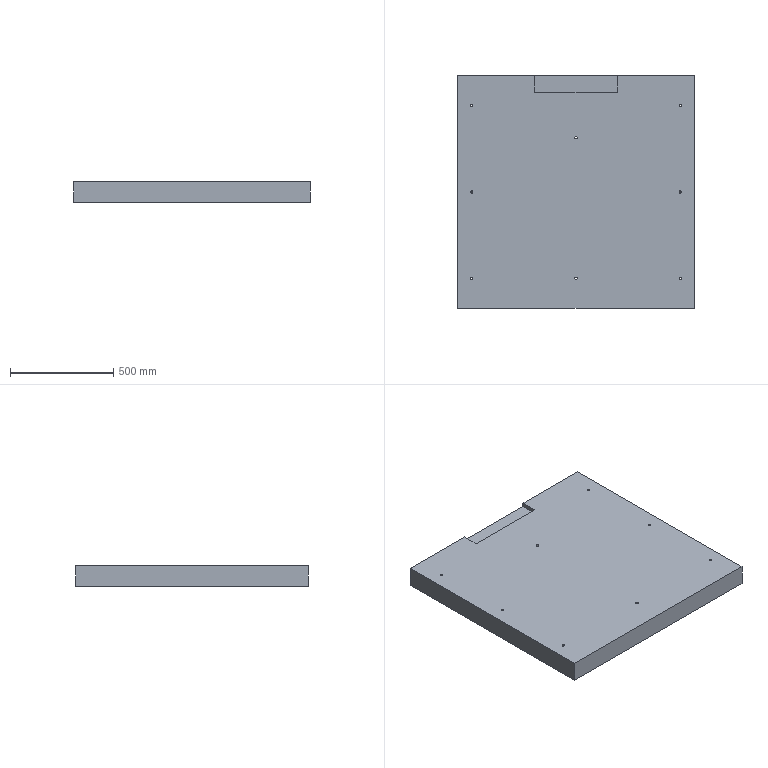Part | SolidWorks | features ICE 3, Extrusion 1 | 1 solid | 26 faces | box 1145 x 1125 x 100 mm | volume 128094667 mm3 | cylinder 16 | plane 10 | commonest cylinder face diameters 11 x14 12 x2
STEP:
#1=CARTESIAN_POINT('',(-6.,262.5,0.));
#2=VERTEX_POINT('',#1);
#3=CARTESIAN_POINT('',(6.,262.5,0.));
#4=VERTEX_POINT('',#3);
#5=CARTESIAN_POINT('',(0.,262.5,0.));
#6=DIRECTION('',(0.,0.,1.));
#7=DIRECTION('',(1.,0.,0.));
#8=AXIS2_PLACEMENT_3D('',#5,#6,#7);
#9=CIRCLE('',#8,6.);
#10=EDGE_CURVE('',#2,#4,#9,.T.);
#11=ORIENTED_EDGE('',*,*,#10,.F.);
#12=CARTESIAN_POINT('',(-6.,262.5,100.));
#13=VERTEX_POINT('',#12);
#14=CARTESIAN_POINT('',(-6.,262.5,0.));
#15=DIRECTION('',(0.,0.,1.));
#16=VECTOR('',#15,1000.);
#17=LINE('',#14,#16);
#18=EDGE_CURVE('',#2,#13,#17,.T.);
#19=ORIENTED_EDGE('',*,*,#18,.T.);
#20=CARTESIAN_POINT('',(6.,262.5,100.));
#21=VERTEX_POINT('',#20);
#22=CARTESIAN_POINT('',(0.,262.5,100.));
#23=DIRECTION('',(0.,0.,1.));
#24=DIRECTION('',(1.,0.,0.));
#25=AXIS2_PLACEMENT_3D('',#22,#23,#24);
#26=CIRCLE('',#25,6.);
#27=EDGE_CURVE('',#13,#21,#26,.T.);
#28=ORIENTED_EDGE('',*,*,#27,.T.);
#29=CARTESIAN_POINT('',(6.,262.5,0.));
#30=DIRECTION('',(0.,0.,1.));
#31=VECTOR('',#30,1000.);
#32=LINE('',#29,#31);
#33=EDGE_CURVE('',#4,#21,#32,.T.);
#34=ORIENTED_EDGE('',*,*,#33,.F.);
#35=EDGE_LOOP('',(#11,#19,#28,#34));
#36=FACE_OUTER_BOUND('',#35,.T.);
#37=CARTESIAN_POINT('',(0.,262.5,0.));
#38=DIRECTION('',(0.,0.,1.));
#39=DIRECTION('',(1.,0.,0.));
#40=AXIS2_PLACEMENT_3D('',#37,#38,#39);
#41=CYLINDRICAL_SURFACE('',#40,6.);
#42=ADVANCED_FACE('',(#36),#41,.F.);
#43=CARTESIAN_POINT('',(-5.5,-417.5,0.));
#44=VERTEX_POINT('',#43);
#45=CARTESIAN_POINT('',(5.5,-417.5,0.));
#46=VERTEX_POINT('',#45);
#47=CARTESIAN_POINT('',(0.,-417.5,0.));
#48=DIRECTION('',(0.,0.,1.));
#49=DIRECTION('',(1.,0.,0.));
#50=AXIS2_PLACEMENT_3D('',#47,#48,#49);
#51=CIRCLE('',#50,5.5);
#52=EDGE_CURVE('',#44,#46,#51,.T.);
#53=ORIENTED_EDGE('',*,*,#52,.F.);
#54=CARTESIAN_POINT('',(-5.5,-417.5,100.));
#55=VERTEX_POINT('',#54);
#56=CARTESIAN_POINT('',(-5.5,-417.5,0.));
#57=DIRECTION('',(0.,0.,1.));
#58=VECTOR('',#57,1000.);
#59=LINE('',#56,#58);
#60=EDGE_CURVE('',#44,#55,#59,.T.);
#61=ORIENTED_EDGE('',*,*,#60,.T.);
#62=CARTESIAN_POINT('',(5.5,-417.5,100.));
#63=VERTEX_POINT('',#62);
#64=CARTESIAN_POINT('',(0.,-417.5,100.));
#65=DIRECTION('',(0.,0.,1.));
#66=DIRECTION('',(1.,0.,0.));
#67=AXIS2_PLACEMENT_3D('',#64,#65,#66);
#68=CIRCLE('',#67,5.5);
#69=EDGE_CURVE('',#55,#63,#68,.T.);
#70=ORIENTED_EDGE('',*,*,#69,.T.);
#71=CARTESIAN_POINT('',(5.5,-417.5,0.));
#72=DIRECTION('',(0.,0.,1.));
#73=VECTOR('',#72,1000.);
#74=LINE('',#71,#73);
#75=EDGE_CURVE('',#46,#63,#74,.T.);
#76=ORIENTED_EDGE('',*,*,#75,.F.);
#77=EDGE_LOOP('',(#53,#61,#70,#76));
#78=FACE_OUTER_BOUND('',#77,.T.);
#79=CARTESIAN_POINT('',(0.,-417.5,0.));
#80=DIRECTION('',(0.,0.,1.));
#81=DIRECTION('',(1.,0.,0.));
#82=AXIS2_PLACEMENT_3D('',#79,#80,#81);
#83=CYLINDRICAL_SURFACE('',#82,5.5);
#84=ADVANCED_FACE('',(#78),#83,.F.);
#85=CARTESIAN_POINT('',(499.,417.5,0.));
#86=VERTEX_POINT('',#85);
#87=CARTESIAN_POINT('',(510.,417.5,0.));
#88=VERTEX_POINT('',#87);
#89=CARTESIAN_POINT('',(504.5,417.5,0.));
#90=DIRECTION('',(0.,0.,1.));
#91=DIRECTION('',(-1.,0.,0.));
#92=AXIS2_PLACEMENT_3D('',#89,#90,#91);
#93=CIRCLE('',#92,5.5);
#94=EDGE_CURVE('',#86,#88,#93,.T.);
#95=ORIENTED_EDGE('',*,*,#94,.F.);
#96=CARTESIAN_POINT('',(499.,417.5,100.));
#97=VERTEX_POINT('',#96);
#98=CARTESIAN_POINT('',(499.,417.5,0.));
#99=DIRECTION('',(0.,0.,1.));
#100=VECTOR('',#99,1000.);
#101=LINE('',#98,#100);
#102=EDGE_CURVE('',#86,#97,#101,.T.);
#103=ORIENTED_EDGE('',*,*,#102,.T.);
#104=CARTESIAN_POINT('',(510.,417.5,100.));
#105=VERTEX_POINT('',#104);
#106=CARTESIAN_POINT('',(504.5,417.5,100.));
#107=DIRECTION('',(0.,0.,1.));
#108=DIRECTION('',(1.,0.,0.));
#109=AXIS2_PLACEMENT_3D('',#106,#107,#108);
#110=CIRCLE('',#109,5.5);
#111=EDGE_CURVE('',#97,#105,#110,.T.);
#112=ORIENTED_EDGE('',*,*,#111,.T.);
#113=CARTESIAN_POINT('',(510.,417.5,0.));
#114=DIRECTION('',(0.,0.,1.));
#115=VECTOR('',#114,1000.);
#116=LINE('',#113,#115);
#117=EDGE_CURVE('',#88,#105,#116,.T.);
#118=ORIENTED_EDGE('',*,*,#117,.F.);
#119=EDGE_LOOP('',(#95,#103,#112,#118));
#120=FACE_OUTER_BOUND('',#119,.T.);
#121=CARTESIAN_POINT('',(504.5,417.5,0.));
#122=DIRECTION('',(0.,0.,1.));
#123=DIRECTION('',(1.,0.,0.));
#124=AXIS2_PLACEMENT_3D('',#121,#122,#123);
#125=CYLINDRICAL_SURFACE('',#124,5.5);
#126=ADVANCED_FACE('',(#120),#125,.F.);
#127=CARTESIAN_POINT('',(499.,-417.5,0.));
#128=VERTEX_POINT('',#127);
#129=CARTESIAN_POINT('',(510.,-417.5,0.));
#130=VERTEX_POINT('',#129);
#131=CARTESIAN_POINT('',(504.5,-417.5,0.));
#132=DIRECTION('',(0.,0.,1.));
#133=DIRECTION('',(-1.,0.,0.));
#134=AXIS2_PLACEMENT_3D('',#131,#132,#133);
#135=CIRCLE('',#134,5.5);
#136=EDGE_CURVE('',#128,#130,#135,.T.);
#137=ORIENTED_EDGE('',*,*,#136,.F.);
#138=CARTESIAN_POINT('',(499.,-417.5,100.));
#139=VERTEX_POINT('',#138);
#140=CARTESIAN_POINT('',(499.,-417.5,0.));
#141=DIRECTION('',(0.,0.,1.));
#142=VECTOR('',#141,1000.);
#143=LINE('',#140,#142);
#144=EDGE_CURVE('',#128,#139,#143,.T.);
#145=ORIENTED_EDGE('',*,*,#144,.T.);
#146=CARTESIAN_POINT('',(510.,-417.5,100.));
#147=VERTEX_POINT('',#146);
#148=CARTESIAN_POINT('',(504.5,-417.5,100.));
#149=DIRECTION('',(0.,0.,1.));
#150=DIRECTION('',(1.,0.,0.));
#151=AXIS2_PLACEMENT_3D('',#148,#149,#150);
#152=CIRCLE('',#151,5.5);
#153=EDGE_CURVE('',#139,#147,#152,.T.);
#154=ORIENTED_EDGE('',*,*,#153,.T.);
#155=CARTESIAN_POINT('',(510.,-417.5,0.));
#156=DIRECTION('',(0.,0.,1.));
#157=VECTOR('',#156,1000.);
#158=LINE('',#155,#157);
#159=EDGE_CURVE('',#130,#147,#158,.T.);
#160=ORIENTED_EDGE('',*,*,#159,.F.);
#161=EDGE_LOOP('',(#137,#145,#154,#160));
#162=FACE_OUTER_BOUND('',#161,.T.);
#163=CARTESIAN_POINT('',(504.5,-417.5,0.));
#164=DIRECTION('',(0.,0.,1.));
#165=DIRECTION('',(1.,0.,0.));
#166=AXIS2_PLACEMENT_3D('',#163,#164,#165);
#167=CYLINDRICAL_SURFACE('',#166,5.5);
#168=ADVANCED_FACE('',(#162),#167,.F.);
#169=CARTESIAN_POINT('',(-510.,-417.5,0.));
#170=VERTEX_POINT('',#169);
#171=CARTESIAN_POINT('',(-499.,-417.5,0.));
#172=VERTEX_POINT('',#171);
#173=CARTESIAN_POINT('',(-504.5,-417.5,0.));
#174=DIRECTION('',(0.,0.,1.));
#175=DIRECTION('',(1.,0.,0.));
#176=AXIS2_PLACEMENT_3D('',#173,#174,#175);
#177=CIRCLE('',#176,5.5);
#178=EDGE_CURVE('',#170,#172,#177,.T.);
#179=ORIENTED_EDGE('',*,*,#178,.F.);
#180=CARTESIAN_POINT('',(-510.,-417.5,100.));
#181=VERTEX_POINT('',#180);
#182=CARTESIAN_POINT('',(-510.,-417.5,0.));
#183=DIRECTION('',(0.,0.,1.));
#184=VECTOR('',#183,1000.);
#185=LINE('',#182,#184);
#186=EDGE_CURVE('',#170,#181,#185,.T.);
#187=ORIENTED_EDGE('',*,*,#186,.T.);
#188=CARTESIAN_POINT('',(-499.,-417.5,100.));
#189=VERTEX_POINT('',#188);
#190=CARTESIAN_POINT('',(-504.5,-417.5,100.));
#191=DIRECTION('',(0.,0.,1.));
#192=DIRECTION('',(1.,0.,0.));
#193=AXIS2_PLACEMENT_3D('',#190,#191,#192);
#194=CIRCLE('',#193,5.5);
#195=EDGE_CURVE('',#181,#189,#194,.T.);
#196=ORIENTED_EDGE('',*,*,#195,.T.);
#197=CARTESIAN_POINT('',(-499.,-417.5,0.));
#198=DIRECTION('',(0.,0.,1.));
#199=VECTOR('',#198,1000.);
#200=LINE('',#197,#199);
#201=EDGE_CURVE('',#172,#189,#200,.T.);
#202=ORIENTED_EDGE('',*,*,#201,.F.);
#203=EDGE_LOOP('',(#179,#187,#196,#202));
#204=FACE_OUTER_BOUND('',#203,.T.);
#205=CARTESIAN_POINT('',(-504.5,-417.5,0.));
#206=DIRECTION('',(0.,0.,1.));
#207=DIRECTION('',(1.,0.,0.));
#208=AXIS2_PLACEMENT_3D('',#205,#206,#207);
#209=CYLINDRICAL_SURFACE('',#208,5.5);
#210=ADVANCED_FACE('',(#204),#209,.F.);
#211=CARTESIAN_POINT('',(-510.,0.,0.));
#212=VERTEX_POINT('',#211);
#213=CARTESIAN_POINT('',(-499.,0.,0.));
#214=VERTEX_POINT('',#213);
#215=CARTESIAN_POINT('',(-504.5,0.,0.));
#216=DIRECTION('',(0.,0.,1.));
#217=DIRECTION('',(1.,0.,0.));
#218=AXIS2_PLACEMENT_3D('',#215,#216,#217);
#219=CIRCLE('',#218,5.5);
#220=EDGE_CURVE('',#212,#214,#219,.T.);
#221=ORIENTED_EDGE('',*,*,#220,.F.);
#222=CARTESIAN_POINT('',(-510.,0.,100.));
#223=VERTEX_POINT('',#222);
#224=CARTESIAN_POINT('',(-510.,0.,0.));
#225=DIRECTION('',(0.,0.,1.));
#226=VECTOR('',#225,1000.);
#227=LINE('',#224,#226);
#228=EDGE_CURVE('',#212,#223,#227,.T.);
#229=ORIENTED_EDGE('',*,*,#228,.T.);
#230=CARTESIAN_POINT('',(-499.,0.,100.));
#231=VERTEX_POINT('',#230);
#232=CARTESIAN_POINT('',(-504.5,0.,100.));
#233=DIRECTION('',(0.,0.,1.));
#234=DIRECTION('',(1.,0.,0.));
#235=AXIS2_PLACEMENT_3D('',#232,#233,#234);
#236=CIRCLE('',#235,5.5);
#237=EDGE_CURVE('',#223,#231,#236,.T.);
#238=ORIENTED_EDGE('',*,*,#237,.T.);
#239=CARTESIAN_POINT('',(-499.,0.,0.));
#240=DIRECTION('',(0.,0.,1.));
#241=VECTOR('',#240,1000.);
#242=LINE('',#239,#241);
#243=EDGE_CURVE('',#214,#231,#242,.T.);
#244=ORIENTED_EDGE('',*,*,#243,.F.);
#245=EDGE_LOOP('',(#221,#229,#238,#244));
#246=FACE_OUTER_BOUND('',#245,.T.);
#247=CARTESIAN_POINT('',(-504.5,0.,0.));
#248=DIRECTION('',(0.,0.,1.));
#249=DIRECTION('',(1.,0.,0.));
#250=AXIS2_PLACEMENT_3D('',#247,#248,#249);
#251=CYLINDRICAL_SURFACE('',#250,5.5);
#252=ADVANCED_FACE('',(#246),#251,.F.);
#253=CARTESIAN_POINT('',(499.,0.,0.));
#254=VERTEX_POINT('',#253);
#255=CARTESIAN_POINT('',(510.,0.,0.));
#256=VERTEX_POINT('',#255);
#257=CARTESIAN_POINT('',(504.5,0.,0.));
#258=DIRECTION('',(0.,0.,1.));
#259=DIRECTION('',(-1.,0.,0.));
#260=AXIS2_PLACEMENT_3D('',#257,#258,#259);
#261=CIRCLE('',#260,5.5);
#262=EDGE_CURVE('',#254,#256,#261,.T.);
#263=ORIENTED_EDGE('',*,*,#262,.F.);
#264=CARTESIAN_POINT('',(499.,0.,100.));
#265=VERTEX_POINT('',#264);
#266=CARTESIAN_POINT('',(499.,0.,0.));
#267=DIRECTION('',(0.,0.,1.));
#268=VECTOR('',#267,1000.);
#269=LINE('',#266,#268);
#270=EDGE_CURVE('',#254,#265,#269,.T.);
#271=ORIENTED_EDGE('',*,*,#270,.T.);
#272=CARTESIAN_POINT('',(510.,0.,100.));
#273=VERTEX_POINT('',#272);
#274=CARTESIAN_POINT('',(504.5,0.,100.));
#275=DIRECTION('',(0.,0.,1.));
#276=DIRECTION('',(1.,0.,0.));
#277=AXIS2_PLACEMENT_3D('',#274,#275,#276);
#278=CIRCLE('',#277,5.5);
#279=EDGE_CURVE('',#265,#273,#278,.T.);
#280=ORIENTED_EDGE('',*,*,#279,.T.);
#281=CARTESIAN_POINT('',(510.,0.,0.));
#282=DIRECTION('',(0.,0.,1.));
#283=VECTOR('',#282,1000.);
#284=LINE('',#281,#283);
#285=EDGE_CURVE('',#256,#273,#284,.T.);
#286=ORIENTED_EDGE('',*,*,#285,.F.);
#287=EDGE_LOOP('',(#263,#271,#280,#286));
#288=FACE_OUTER_BOUND('',#287,.T.);
#289=CARTESIAN_POINT('',(504.5,0.,0.));
#290=DIRECTION('',(0.,0.,1.));
#291=DIRECTION('',(1.,0.,0.));
#292=AXIS2_PLACEMENT_3D('',#289,#290,#291);
#293=CYLINDRICAL_SURFACE('',#292,5.5);
#294=ADVANCED_FACE('',(#288),#293,.F.);
#295=CARTESIAN_POINT('',(-510.,417.5,0.));
#296=VERTEX_POINT('',#295);
#297=CARTESIAN_POINT('',(-499.,417.5,0.));
#298=VERTEX_POINT('',#297);
#299=CARTESIAN_POINT('',(-504.5,417.5,0.));
#300=DIRECTION('',(0.,0.,1.));
#301=DIRECTION('',(1.,0.,0.));
#302=AXIS2_PLACEMENT_3D('',#299,#300,#301);
#303=CIRCLE('',#302,5.5);
#304=EDGE_CURVE('',#296,#298,#303,.T.);
#305=ORIENTED_EDGE('',*,*,#304,.F.);
#306=CARTESIAN_POINT('',(-510.,417.5,100.));
#307=VERTEX_POINT('',#306);
#308=CARTESIAN_POINT('',(-510.,417.5,0.));
#309=DIRECTION('',(0.,0.,1.));
#310=VECTOR('',#309,1000.);
#311=LINE('',#308,#310);
#312=EDGE_CURVE('',#296,#307,#311,.T.);
#313=ORIENTED_EDGE('',*,*,#312,.T.);
#314=CARTESIAN_POINT('',(-499.,417.5,100.));
#315=VERTEX_POINT('',#314);
#316=CARTESIAN_POINT('',(-504.5,417.5,100.));
#317=DIRECTION('',(0.,0.,1.));
#318=DIRECTION('',(1.,0.,0.));
#319=AXIS2_PLACEMENT_3D('',#316,#317,#318);
#320=CIRCLE('',#319,5.5);
#321=EDGE_CURVE('',#307,#315,#320,.T.);
#322=ORIENTED_EDGE('',*,*,#321,.T.);
#323=CARTESIAN_POINT('',(-499.,417.5,0.));
#324=DIRECTION('',(0.,0.,1.));
#325=VECTOR('',#324,1000.);
#326=LINE('',#323,#325);
#327=EDGE_CURVE('',#298,#315,#326,.T.);
#328=ORIENTED_EDGE('',*,*,#327,.F.);
#329=EDGE_LOOP('',(#305,#313,#322,#328));
#330=FACE_OUTER_BOUND('',#329,.T.);
#331=CARTESIAN_POINT('',(-504.5,417.5,0.));
#332=DIRECTION('',(0.,0.,1.));
#333=DIRECTION('',(1.,0.,0.));
#334=AXIS2_PLACEMENT_3D('',#331,#332,#333);
#335=CYLINDRICAL_SURFACE('',#334,5.5);
#336=ADVANCED_FACE('',(#330),#335,.F.);
#337=CARTESIAN_POINT('',(572.5,-562.5,0.));
#338=VERTEX_POINT('',#337);
#339=CARTESIAN_POINT('',(572.5,562.5,0.));
#340=VERTEX_POINT('',#339);
#341=CARTESIAN_POINT('',(572.5,562.5,0.));
#342=DIRECTION('',(0.,1.,0.));
#343=VECTOR('',#342,1000.);
#344=LINE('',#341,#343);
#345=EDGE_CURVE('',#338,#340,#344,.T.);
#346=ORIENTED_EDGE('',*,*,#345,.T.);
#347=CARTESIAN_POINT('',(572.5,562.5,100.));
#348=VERTEX_POINT('',#347);
#349=CARTESIAN_POINT('',(572.5,562.5,100.));
#350=DIRECTION('',(0.,0.,-1.));
#351=VECTOR('',#350,1000.);
#352=LINE('',#349,#351);
#353=EDGE_CURVE('',#348,#340,#352,.T.);
#354=ORIENTED_EDGE('',*,*,#353,.F.);
#355=CARTESIAN_POINT('',(572.5,-562.5,100.));
#356=VERTEX_POINT('',#355);
#357=CARTESIAN_POINT('',(572.5,562.5,100.));
#358=DIRECTION('',(0.,1.,0.));
#359=VECTOR('',#358,1000.);
#360=LINE('',#357,#359);
#361=EDGE_CURVE('',#356,#348,#360,.T.);
#362=ORIENTED_EDGE('',*,*,#361,.F.);
#363=CARTESIAN_POINT('',(572.5,-562.5,100.));
#364=DIRECTION('',(0.,0.,-1.));
#365=VECTOR('',#364,1000.);
#366=LINE('',#363,#365);
#367=EDGE_CURVE('',#356,#338,#366,.T.);
#368=ORIENTED_EDGE('',*,*,#367,.T.);
#369=EDGE_LOOP('',(#346,#354,#362,#368));
#370=FACE_OUTER_BOUND('',#369,.T.);
#371=CARTESIAN_POINT('',(572.5,562.5,100.));
#372=DIRECTION('',(-1.,0.,0.));
#373=DIRECTION('',(0.,-1.,0.));
#374=AXIS2_PLACEMENT_3D('',#371,#372,#373);
#375=PLANE('',#374);
#376=ADVANCED_FACE('',(#370),#375,.F.);
#377=CARTESIAN_POINT('',(200.,562.5,80.));
#378=VERTEX_POINT('',#377);
#379=CARTESIAN_POINT('',(-200.,562.5,80.));
#380=VERTEX_POINT('',#379);
#381=CARTESIAN_POINT('',(-572.5,562.5,80.));
#382=DIRECTION('',(-1.,0.,0.));
#383=VECTOR('',#382,1000.);
#384=LINE('',#381,#383);
#385=EDGE_CURVE('',#378,#380,#384,.T.);
#386=ORIENTED_EDGE('',*,*,#385,.F.);
#387=CARTESIAN_POINT('',(200.,562.5,100.));
#388=VERTEX_POINT('',#387);
#389=CARTESIAN_POINT('',(200.,562.5,100.));
#390=DIRECTION('',(0.,0.,1.));
#391=VECTOR('',#390,1000.);
#392=LINE('',#389,#391);
#393=EDGE_CURVE('',#378,#388,#392,.T.);
#394=ORIENTED_EDGE('',*,*,#393,.T.);
#395=CARTESIAN_POINT('',(-572.5,562.5,100.));
#396=DIRECTION('',(-1.,0.,0.));
#397=VECTOR('',#396,1000.);
#398=LINE('',#395,#397);
#399=EDGE_CURVE('',#348,#388,#398,.T.);
#400=ORIENTED_EDGE('',*,*,#399,.F.);
#401=ORIENTED_EDGE('',*,*,#353,.T.);
#402=CARTESIAN_POINT('',(-572.5,562.5,0.));
#403=VERTEX_POINT('',#402);
#404=CARTESIAN_POINT('',(-572.5,562.5,0.));
#405=DIRECTION('',(-1.,0.,0.));
#406=VECTOR('',#405,1000.);
#407=LINE('',#404,#406);
#408=EDGE_CURVE('',#340,#403,#407,.T.);
#409=ORIENTED_EDGE('',*,*,#408,.T.);
#410=CARTESIAN_POINT('',(-572.5,562.5,100.));
#411=VERTEX_POINT('',#410);
#412=CARTESIAN_POINT('',(-572.5,562.5,100.));
#413=DIRECTION('',(0.,0.,-1.));
#414=VECTOR('',#413,1000.);
#415=LINE('',#412,#414);
#416=EDGE_CURVE('',#411,#403,#415,.T.);
#417=ORIENTED_EDGE('',*,*,#416,.F.);
#418=CARTESIAN_POINT('',(-200.,562.5,100.));
#419=VERTEX_POINT('',#418);
#420=CARTESIAN_POINT('',(-572.5,562.5,100.));
#421=DIRECTION('',(-1.,0.,0.));
#422=VECTOR('',#421,1000.);
#423=LINE('',#420,#422);
#424=EDGE_CURVE('',#419,#411,#423,.T.);
#425=ORIENTED_EDGE('',*,*,#424,.F.);
#426=CARTESIAN_POINT('',(-200.,562.5,100.));
#427=DIRECTION('',(0.,0.,-1.));
#428=VECTOR('',#427,1000.);
#429=LINE('',#426,#428);
#430=EDGE_CURVE('',#419,#380,#429,.T.);
#431=ORIENTED_EDGE('',*,*,#430,.T.);
#432=EDGE_LOOP('',(#386,#394,#400,#401,#409,#417,#425,#431));
#433=FACE_OUTER_BOUND('',#432,.T.);
#434=CARTESIAN_POINT('',(-572.5,562.5,100.));
#435=DIRECTION('',(0.,-1.,0.));
#436=DIRECTION('',(0.,0.,-1.));
#437=AXIS2_PLACEMENT_3D('',#434,#435,#436);
#438=PLANE('',#437);
#439=ADVANCED_FACE('',(#433),#438,.F.);
#440=CARTESIAN_POINT('',(-572.5,-562.5,0.));
#441=VERTEX_POINT('',#440);
#442=CARTESIAN_POINT('',(-572.5,562.5,0.));
#443=DIRECTION('',(0.,-1.,0.));
#444=VECTOR('',#443,1000.);
#445=LINE('',#442,#444);
#446=EDGE_CURVE('',#403,#441,#445,.T.);
#447=ORIENTED_EDGE('',*,*,#446,.T.);
#448=CARTESIAN_POINT('',(-572.5,-562.5,100.));
#449=VERTEX_POINT('',#448);
#450=CARTESIAN_POINT('',(-572.5,-562.5,100.));
#451=DIRECTION('',(0.,0.,-1.));
#452=VECTOR('',#451,1000.);
#453=LINE('',#450,#452);
#454=EDGE_CURVE('',#449,#441,#453,.T.);
#455=ORIENTED_EDGE('',*,*,#454,.F.);
#456=CARTESIAN_POINT('',(-572.5,562.5,100.));
#457=DIRECTION('',(0.,-1.,0.));
#458=VECTOR('',#457,1000.);
#459=LINE('',#456,#458);
#460=EDGE_CURVE('',#411,#449,#459,.T.);
#461=ORIENTED_EDGE('',*,*,#460,.F.);
#462=ORIENTED_EDGE('',*,*,#416,.T.);
#463=EDGE_LOOP('',(#447,#455,#461,#462));
#464=FACE_OUTER_BOUND('',#463,.T.);
#465=CARTESIAN_POINT('',(-572.5,562.5,100.));
#466=DIRECTION('',(1.,0.,0.));
#467=DIRECTION('',(0.,1.,0.));
#468=AXIS2_PLACEMENT_3D('',#465,#466,#467);
#469=PLANE('',#468);
#470=ADVANCED_FACE('',(#464),#469,.F.);
#471=CARTESIAN_POINT('',(-572.5,-562.5,0.));
#472=DIRECTION('',(1.,0.,0.));
#473=VECTOR('',#472,1000.);
#474=LINE('',#471,#473);
#475=EDGE_CURVE('',#441,#338,#474,.T.);
#476=ORIENTED_EDGE('',*,*,#475,.T.);
#477=ORIENTED_EDGE('',*,*,#367,.F.);
#478=CARTESIAN_POINT('',(-572.5,-562.5,100.));
#479=DIRECTION('',(1.,0.,0.));
#480=VECTOR('',#479,1000.);
#481=LINE('',#478,#480);
#482=EDGE_CURVE('',#449,#356,#481,.T.);
#483=ORIENTED_EDGE('',*,*,#482,.F.);
#484=ORIENTED_EDGE('',*,*,#454,.T.);
#485=EDGE_LOOP('',(#476,#477,#483,#484));
#486=FACE_OUTER_BOUND('',#485,.T.);
#487=CARTESIAN_POINT('',(-572.5,-562.5,100.));
#488=DIRECTION('',(0.,1.,0.));
#489=DIRECTION('',(0.,0.,1.));
#490=AXIS2_PLACEMENT_3D('',#487,#488,#489);
#491=PLANE('',#490);
#492=ADVANCED_FACE('',(#486),#491,.F.);
#493=CARTESIAN_POINT('',(0.,262.5,100.));
#494=DIRECTION('',(0.,0.,1.));
#495=DIRECTION('',(1.,0.,0.));
#496=AXIS2_PLACEMENT_3D('',#493,#494,#495);
#497=CIRCLE('',#496,6.);
#498=EDGE_CURVE('',#21,#13,#497,.T.);
#499=ORIENTED_EDGE('',*,*,#498,.F.);
#500=ORIENTED_EDGE('',*,*,#27,.F.);
#501=EDGE_LOOP('',(#499,#500));
#502=FACE_BOUND('',#501,.T.);
#503=CARTESIAN_POINT('',(0.,-417.5,100.));
#504=DIRECTION('',(0.,0.,1.));
#505=DIRECTION('',(1.,0.,0.));
#506=AXIS2_PLACEMENT_3D('',#503,#504,#505);
#507=CIRCLE('',#506,5.5);
#508=EDGE_CURVE('',#63,#55,#507,.T.);
#509=ORIENTED_EDGE('',*,*,#508,.F.);
#510=ORIENTED_EDGE('',*,*,#69,.F.);
#511=EDGE_LOOP('',(#509,#510));
#512=FACE_BOUND('',#511,.T.);
#513=CARTESIAN_POINT('',(504.5,417.5,100.));
#514=DIRECTION('',(0.,0.,1.));
#515=DIRECTION('',(1.,0.,0.));
#516=AXIS2_PLACEMENT_3D('',#513,#514,#515);
#517=CIRCLE('',#516,5.5);
#518=EDGE_CURVE('',#105,#97,#517,.T.);
#519=ORIENTED_EDGE('',*,*,#518,.F.);
#520=ORIENTED_EDGE('',*,*,#111,.F.);
#521=EDGE_LOOP('',(#519,#520));
#522=FACE_BOUND('',#521,.T.);
#523=CARTESIAN_POINT('',(504.5,-417.5,100.));
#524=DIRECTION('',(0.,0.,1.));
#525=DIRECTION('',(1.,0.,0.));
#526=AXIS2_PLACEMENT_3D('',#523,#524,#525);
#527=CIRCLE('',#526,5.5);
#528=EDGE_CURVE('',#147,#139,#527,.T.);
#529=ORIENTED_EDGE('',*,*,#528,.F.);
#530=ORIENTED_EDGE('',*,*,#153,.F.);
#531=EDGE_LOOP('',(#529,#530));
#532=FACE_BOUND('',#531,.T.);
#533=CARTESIAN_POINT('',(-504.5,-417.5,100.));
#534=DIRECTION('',(0.,0.,1.));
#535=DIRECTION('',(1.,0.,0.));
#536=AXIS2_PLACEMENT_3D('',#533,#534,#535);
#537=CIRCLE('',#536,5.5);
#538=EDGE_CURVE('',#189,#181,#537,.T.);
#539=ORIENTED_EDGE('',*,*,#538,.F.);
#540=ORIENTED_EDGE('',*,*,#195,.F.);
#541=EDGE_LOOP('',(#539,#540));
#542=FACE_BOUND('',#541,.T.);
#543=CARTESIAN_POINT('',(-504.5,0.,100.));
#544=DIRECTION('',(0.,0.,1.));
#545=DIRECTION('',(1.,0.,0.));
#546=AXIS2_PLACEMENT_3D('',#543,#544,#545);
#547=CIRCLE('',#546,5.5);
#548=EDGE_CURVE('',#231,#223,#547,.T.);
#549=ORIENTED_EDGE('',*,*,#548,.F.);
#550=ORIENTED_EDGE('',*,*,#237,.F.);
#551=EDGE_LOOP('',(#549,#550));
#552=FACE_BOUND('',#551,.T.);
#553=CARTESIAN_POINT('',(504.5,0.,100.));
#554=DIRECTION('',(0.,0.,1.));
#555=DIRECTION('',(1.,0.,0.));
#556=AXIS2_PLACEMENT_3D('',#553,#554,#555);
#557=CIRCLE('',#556,5.5);
#558=EDGE_CURVE('',#273,#265,#557,.T.);
#559=ORIENTED_EDGE('',*,*,#558,.F.);
#560=ORIENTED_EDGE('',*,*,#279,.F.);
#561=EDGE_LOOP('',(#559,#560));
#562=FACE_BOUND('',#561,.T.);
#563=CARTESIAN_POINT('',(-504.5,417.5,100.));
#564=DIRECTION('',(0.,0.,1.));
#565=DIRECTION('',(1.,0.,0.));
#566=AXIS2_PLACEMENT_3D('',#563,#564,#565);
#567=CIRCLE('',#566,5.5);
#568=EDGE_CURVE('',#315,#307,#567,.T.);
#569=ORIENTED_EDGE('',*,*,#568,.F.);
#570=ORIENTED_EDGE('',*,*,#321,.F.);
#571=EDGE_LOOP('',(#569,#570));
#572=FACE_BOUND('',#571,.T.);
#573=CARTESIAN_POINT('',(200.,482.5,100.));
#574=VERTEX_POINT('',#573);
#575=CARTESIAN_POINT('',(200.,642.5,100.));
#576=DIRECTION('',(0.,1.,0.));
#577=VECTOR('',#576,1000.);
#578=LINE('',#575,#577);
#579=EDGE_CURVE('',#574,#388,#578,.T.);
#580=ORIENTED_EDGE('',*,*,#579,.F.);
#581=CARTESIAN_POINT('',(-200.,482.5,100.));
#582=VERTEX_POINT('',#581);
#583=CARTESIAN_POINT('',(-200.,482.5,100.));
#584=DIRECTION('',(1.,0.,0.));
#585=VECTOR('',#584,1000.);
#586=LINE('',#583,#585);
#587=EDGE_CURVE('',#582,#574,#586,.T.);
#588=ORIENTED_EDGE('',*,*,#587,.F.);
#589=CARTESIAN_POINT('',(-200.,0.,100.));
#590=DIRECTION('',(0.,-1.,0.));
#591=VECTOR('',#590,1000.);
#592=LINE('',#589,#591);
#593=EDGE_CURVE('',#419,#582,#592,.T.);
#594=ORIENTED_EDGE('',*,*,#593,.F.);
#595=ORIENTED_EDGE('',*,*,#424,.T.);
#596=ORIENTED_EDGE('',*,*,#460,.T.);
#597=ORIENTED_EDGE('',*,*,#482,.T.);
#598=ORIENTED_EDGE('',*,*,#361,.T.);
#599=ORIENTED_EDGE('',*,*,#399,.T.);
#600=EDGE_LOOP('',(#580,#588,#594,#595,#596,#597,#598,#599));
#601=FACE_OUTER_BOUND('',#600,.T.);
#602=CARTESIAN_POINT('',(0.,0.,100.));
#603=DIRECTION('',(0.,0.,1.));
#604=DIRECTION('',(1.,0.,0.));
#605=AXIS2_PLACEMENT_3D('',#602,#603,#604);
#606=PLANE('',#605);
#607=ADVANCED_FACE('',(#502,#512,#522,#532,#542,#552,#562,#572,#601),#606,.T.);
#608=CARTESIAN_POINT('',(0.,262.5,0.));
#609=DIRECTION('',(0.,0.,1.));
#610=DIRECTION('',(1.,0.,0.));
#611=AXIS2_PLACEMENT_3D('',#608,#609,#610);
#612=CIRCLE('',#611,6.);
#613=EDGE_CURVE('',#4,#2,#612,.T.);
#614=ORIENTED_EDGE('',*,*,#613,.T.);
#615=ORIENTED_EDGE('',*,*,#10,.T.);
#616=EDGE_LOOP('',(#614,#615));
#617=FACE_BOUND('',#616,.T.);
#618=CARTESIAN_POINT('',(0.,-417.5,0.));
#619=DIRECTION('',(0.,0.,1.));
#620=DIRECTION('',(1.,0.,0.));
#621=AXIS2_PLACEMENT_3D('',#618,#619,#620);
#622=CIRCLE('',#621,5.5);
#623=EDGE_CURVE('',#46,#44,#622,.T.);
#624=ORIENTED_EDGE('',*,*,#623,.T.);
#625=ORIENTED_EDGE('',*,*,#52,.T.);
#626=EDGE_LOOP('',(#624,#625));
#627=FACE_BOUND('',#626,.T.);
#628=CARTESIAN_POINT('',(504.5,417.5,0.));
#629=DIRECTION('',(0.,0.,1.));
#630=DIRECTION('',(-1.,0.,0.));
#631=AXIS2_PLACEMENT_3D('',#628,#629,#630);
#632=CIRCLE('',#631,5.5);
#633=EDGE_CURVE('',#88,#86,#632,.T.);
#634=ORIENTED_EDGE('',*,*,#633,.T.);
#635=ORIENTED_EDGE('',*,*,#94,.T.);
#636=EDGE_LOOP('',(#634,#635));
#637=FACE_BOUND('',#636,.T.);
#638=CARTESIAN_POINT('',(504.5,-417.5,0.));
#639=DIRECTION('',(0.,0.,1.));
#640=DIRECTION('',(-1.,0.,0.));
#641=AXIS2_PLACEMENT_3D('',#638,#639,#640);
#642=CIRCLE('',#641,5.5);
#643=EDGE_CURVE('',#130,#128,#642,.T.);
#644=ORIENTED_EDGE('',*,*,#643,.T.);
#645=ORIENTED_EDGE('',*,*,#136,.T.);
#646=EDGE_LOOP('',(#644,#645));
#647=FACE_BOUND('',#646,.T.);
#648=CARTESIAN_POINT('',(-504.5,-417.5,0.));
#649=DIRECTION('',(0.,0.,1.));
#650=DIRECTION('',(1.,0.,0.));
#651=AXIS2_PLACEMENT_3D('',#648,#649,#650);
#652=CIRCLE('',#651,5.5);
#653=EDGE_CURVE('',#172,#170,#652,.T.);
#654=ORIENTED_EDGE('',*,*,#653,.T.);
#655=ORIENTED_EDGE('',*,*,#178,.T.);
#656=EDGE_LOOP('',(#654,#655));
#657=FACE_BOUND('',#656,.T.);
#658=CARTESIAN_POINT('',(-504.5,0.,0.));
#659=DIRECTION('',(0.,0.,1.));
#660=DIRECTION('',(1.,0.,0.));
#661=AXIS2_PLACEMENT_3D('',#658,#659,#660);
#662=CIRCLE('',#661,5.5);
#663=EDGE_CURVE('',#214,#212,#662,.T.);
#664=ORIENTED_EDGE('',*,*,#663,.T.);
#665=ORIENTED_EDGE('',*,*,#220,.T.);
#666=EDGE_LOOP('',(#664,#665));
#667=FACE_BOUND('',#666,.T.);
#668=CARTESIAN_POINT('',(504.5,0.,0.));
#669=DIRECTION('',(0.,0.,1.));
#670=DIRECTION('',(-1.,0.,0.));
#671=AXIS2_PLACEMENT_3D('',#668,#669,#670);
#672=CIRCLE('',#671,5.5);
#673=EDGE_CURVE('',#256,#254,#672,.T.);
#674=ORIENTED_EDGE('',*,*,#673,.T.);
#675=ORIENTED_EDGE('',*,*,#262,.T.);
#676=EDGE_LOOP('',(#674,#675));
#677=FACE_BOUND('',#676,.T.);
#678=CARTESIAN_POINT('',(-504.5,417.5,0.));
#679=DIRECTION('',(0.,0.,1.));
#680=DIRECTION('',(1.,0.,0.));
#681=AXIS2_PLACEMENT_3D('',#678,#679,#680);
#682=CIRCLE('',#681,5.5);
#683=EDGE_CURVE('',#298,#296,#682,.T.);
#684=ORIENTED_EDGE('',*,*,#683,.T.);
#685=ORIENTED_EDGE('',*,*,#304,.T.);
#686=EDGE_LOOP('',(#684,#685));
#687=FACE_BOUND('',#686,.T.);
#688=ORIENTED_EDGE('',*,*,#345,.F.);
#689=ORIENTED_EDGE('',*,*,#475,.F.);
#690=ORIENTED_EDGE('',*,*,#446,.F.);
#691=ORIENTED_EDGE('',*,*,#408,.F.);
#692=EDGE_LOOP('',(#688,#689,#690,#691));
#693=FACE_OUTER_BOUND('',#692,.T.);
#694=CARTESIAN_POINT('',(0.,0.,0.));
#695=DIRECTION('',(0.,0.,1.));
#696=DIRECTION('',(1.,0.,0.));
#697=AXIS2_PLACEMENT_3D('',#694,#695,#696);
#698=PLANE('',#697);
#699=ADVANCED_FACE('',(#617,#627,#637,#647,#657,#667,#677,#687,#693),#698,.F.);
#700=ORIENTED_EDGE('',*,*,#385,.T.);
#701=CARTESIAN_POINT('',(-200.,482.5,80.));
#702=VERTEX_POINT('',#701);
#703=CARTESIAN_POINT('',(-200.,642.5,80.));
#704=DIRECTION('',(0.,-1.,0.));
#705=VECTOR('',#704,1000.);
#706=LINE('',#703,#705);
#707=EDGE_CURVE('',#380,#702,#706,.T.);
#708=ORIENTED_EDGE('',*,*,#707,.T.);
#709=CARTESIAN_POINT('',(200.,482.5,80.));
#710=VERTEX_POINT('',#709);
#711=CARTESIAN_POINT('',(-200.,482.5,80.));
#712=DIRECTION('',(1.,0.,0.));
#713=VECTOR('',#712,1000.);
#714=LINE('',#711,#713);
#715=EDGE_CURVE('',#702,#710,#714,.T.);
#716=ORIENTED_EDGE('',*,*,#715,.T.);
#717=CARTESIAN_POINT('',(200.,642.5,80.));
#718=DIRECTION('',(0.,1.,0.));
#719=VECTOR('',#718,1000.);
#720=LINE('',#717,#719);
#721=EDGE_CURVE('',#710,#378,#720,.T.);
#722=ORIENTED_EDGE('',*,*,#721,.T.);
#723=EDGE_LOOP('',(#700,#708,#716,#722));
#724=FACE_OUTER_BOUND('',#723,.T.);
#725=CARTESIAN_POINT('',(0.,0.,80.));
#726=DIRECTION('',(0.,0.,1.));
#727=DIRECTION('',(1.,0.,0.));
#728=AXIS2_PLACEMENT_3D('',#725,#726,#727);
#729=PLANE('',#728);
#730=ADVANCED_FACE('',(#724),#729,.T.);
#731=ORIENTED_EDGE('',*,*,#721,.F.);
#732=CARTESIAN_POINT('',(200.,482.5,80.));
#733=DIRECTION('',(0.,0.,1.));
#734=VECTOR('',#733,1000.);
#735=LINE('',#732,#734);
#736=EDGE_CURVE('',#710,#574,#735,.T.);
#737=ORIENTED_EDGE('',*,*,#736,.T.);
#738=ORIENTED_EDGE('',*,*,#579,.T.);
#739=ORIENTED_EDGE('',*,*,#393,.F.);
#740=EDGE_LOOP('',(#731,#737,#738,#739));
#741=FACE_OUTER_BOUND('',#740,.T.);
#742=CARTESIAN_POINT('',(200.,642.5,80.));
#743=DIRECTION('',(1.,0.,0.));
#744=DIRECTION('',(0.,1.,0.));
#745=AXIS2_PLACEMENT_3D('',#742,#743,#744);
#746=PLANE('',#745);
#747=ADVANCED_FACE('',(#741),#746,.F.);
#748=ORIENTED_EDGE('',*,*,#593,.T.);
#749=CARTESIAN_POINT('',(-200.,482.5,80.));
#750=DIRECTION('',(0.,0.,1.));
#751=VECTOR('',#750,1000.);
#752=LINE('',#749,#751);
#753=EDGE_CURVE('',#702,#582,#752,.T.);
#754=ORIENTED_EDGE('',*,*,#753,.F.);
#755=ORIENTED_EDGE('',*,*,#707,.F.);
#756=ORIENTED_EDGE('',*,*,#430,.F.);
#757=EDGE_LOOP('',(#748,#754,#755,#756));
#758=FACE_OUTER_BOUND('',#757,.T.);
#759=CARTESIAN_POINT('',(-200.,642.5,80.));
#760=DIRECTION('',(-1.,0.,0.));
#761=DIRECTION('',(0.,0.,1.));
#762=AXIS2_PLACEMENT_3D('',#759,#760,#761);
#763=PLANE('',#762);
#764=ADVANCED_FACE('',(#758),#763,.F.);
#765=ORIENTED_EDGE('',*,*,#587,.T.);
#766=ORIENTED_EDGE('',*,*,#736,.F.);
#767=ORIENTED_EDGE('',*,*,#715,.F.);
#768=ORIENTED_EDGE('',*,*,#753,.T.);
#769=EDGE_LOOP('',(#765,#766,#767,#768));
#770=FACE_OUTER_BOUND('',#769,.T.);
#771=CARTESIAN_POINT('',(-200.,482.5,80.));
#772=DIRECTION('',(0.,-1.,0.));
#773=DIRECTION('',(0.,0.,-1.));
#774=AXIS2_PLACEMENT_3D('',#771,#772,#773);
#775=PLANE('',#774);
#776=ADVANCED_FACE('',(#770),#775,.F.);
#777=ORIENTED_EDGE('',*,*,#312,.F.);
#778=ORIENTED_EDGE('',*,*,#683,.F.);
#779=ORIENTED_EDGE('',*,*,#327,.T.);
#780=ORIENTED_EDGE('',*,*,#568,.T.);
#781=EDGE_LOOP('',(#777,#778,#779,#780));
#782=FACE_OUTER_BOUND('',#781,.T.);
#783=CARTESIAN_POINT('',(-504.5,417.5,0.));
#784=DIRECTION('',(0.,0.,1.));
#785=DIRECTION('',(1.,0.,0.));
#786=AXIS2_PLACEMENT_3D('',#783,#784,#785);
#787=CYLINDRICAL_SURFACE('',#786,5.5);
#788=ADVANCED_FACE('',(#782),#787,.F.);
#789=ORIENTED_EDGE('',*,*,#270,.F.);
#790=ORIENTED_EDGE('',*,*,#673,.F.);
#791=ORIENTED_EDGE('',*,*,#285,.T.);
#792=ORIENTED_EDGE('',*,*,#558,.T.);
#793=EDGE_LOOP('',(#789,#790,#791,#792));
#794=FACE_OUTER_BOUND('',#793,.T.);
#795=CARTESIAN_POINT('',(504.5,0.,0.));
#796=DIRECTION('',(0.,0.,1.));
#797=DIRECTION('',(1.,0.,0.));
#798=AXIS2_PLACEMENT_3D('',#795,#796,#797);
#799=CYLINDRICAL_SURFACE('',#798,5.5);
#800=ADVANCED_FACE('',(#794),#799,.F.);
#801=ORIENTED_EDGE('',*,*,#228,.F.);
#802=ORIENTED_EDGE('',*,*,#663,.F.);
#803=ORIENTED_EDGE('',*,*,#243,.T.);
#804=ORIENTED_EDGE('',*,*,#548,.T.);
#805=EDGE_LOOP('',(#801,#802,#803,#804));
#806=FACE_OUTER_BOUND('',#805,.T.);
#807=CARTESIAN_POINT('',(-504.5,0.,0.));
#808=DIRECTION('',(0.,0.,1.));
#809=DIRECTION('',(1.,0.,0.));
#810=AXIS2_PLACEMENT_3D('',#807,#808,#809);
#811=CYLINDRICAL_SURFACE('',#810,5.5);
#812=ADVANCED_FACE('',(#806),#811,.F.);
#813=ORIENTED_EDGE('',*,*,#186,.F.);
#814=ORIENTED_EDGE('',*,*,#653,.F.);
#815=ORIENTED_EDGE('',*,*,#201,.T.);
#816=ORIENTED_EDGE('',*,*,#538,.T.);
#817=EDGE_LOOP('',(#813,#814,#815,#816));
#818=FACE_OUTER_BOUND('',#817,.T.);
#819=CARTESIAN_POINT('',(-504.5,-417.5,0.));
#820=DIRECTION('',(0.,0.,1.));
#821=DIRECTION('',(1.,0.,0.));
#822=AXIS2_PLACEMENT_3D('',#819,#820,#821);
#823=CYLINDRICAL_SURFACE('',#822,5.5);
#824=ADVANCED_FACE('',(#818),#823,.F.);
#825=ORIENTED_EDGE('',*,*,#144,.F.);
#826=ORIENTED_EDGE('',*,*,#643,.F.);
#827=ORIENTED_EDGE('',*,*,#159,.T.);
#828=ORIENTED_EDGE('',*,*,#528,.T.);
#829=EDGE_LOOP('',(#825,#826,#827,#828));
#830=FACE_OUTER_BOUND('',#829,.T.);
#831=CARTESIAN_POINT('',(504.5,-417.5,0.));
#832=DIRECTION('',(0.,0.,1.));
#833=DIRECTION('',(1.,0.,0.));
#834=AXIS2_PLACEMENT_3D('',#831,#832,#833);
#835=CYLINDRICAL_SURFACE('',#834,5.5);
#836=ADVANCED_FACE('',(#830),#835,.F.);
#837=ORIENTED_EDGE('',*,*,#102,.F.);
#838=ORIENTED_EDGE('',*,*,#633,.F.);
#839=ORIENTED_EDGE('',*,*,#117,.T.);
#840=ORIENTED_EDGE('',*,*,#518,.T.);
#841=EDGE_LOOP('',(#837,#838,#839,#840));
#842=FACE_OUTER_BOUND('',#841,.T.);
#843=CARTESIAN_POINT('',(504.5,417.5,0.));
#844=DIRECTION('',(0.,0.,1.));
#845=DIRECTION('',(1.,0.,0.));
#846=AXIS2_PLACEMENT_3D('',#843,#844,#845);
#847=CYLINDRICAL_SURFACE('',#846,5.5);
#848=ADVANCED_FACE('',(#842),#847,.F.);
#849=ORIENTED_EDGE('',*,*,#60,.F.);
#850=ORIENTED_EDGE('',*,*,#623,.F.);
#851=ORIENTED_EDGE('',*,*,#75,.T.);
#852=ORIENTED_EDGE('',*,*,#508,.T.);
#853=EDGE_LOOP('',(#849,#850,#851,#852));
#854=FACE_OUTER_BOUND('',#853,.T.);
#855=CARTESIAN_POINT('',(0.,-417.5,0.));
#856=DIRECTION('',(0.,0.,1.));
#857=DIRECTION('',(1.,0.,0.));
#858=AXIS2_PLACEMENT_3D('',#855,#856,#857);
#859=CYLINDRICAL_SURFACE('',#858,5.5);
#860=ADVANCED_FACE('',(#854),#859,.F.);
#861=ORIENTED_EDGE('',*,*,#18,.F.);
#862=ORIENTED_EDGE('',*,*,#613,.F.);
#863=ORIENTED_EDGE('',*,*,#33,.T.);
#864=ORIENTED_EDGE('',*,*,#498,.T.);
#865=EDGE_LOOP('',(#861,#862,#863,#864));
#866=FACE_OUTER_BOUND('',#865,.T.);
#867=CARTESIAN_POINT('',(0.,262.5,0.));
#868=DIRECTION('',(0.,0.,1.));
#869=DIRECTION('',(1.,0.,0.));
#870=AXIS2_PLACEMENT_3D('',#867,#868,#869);
#871=CYLINDRICAL_SURFACE('',#870,6.);
#872=ADVANCED_FACE('',(#866),#871,.F.);
#873=CLOSED_SHELL('',(#42,#84,#126,#168,#210,#252,#294,#336,#376,#439,#470,#492,#607,#699,#730,#747,#764,#776,#788,#800,#812,#824,#836,#848,#860,#872));
#874=MANIFOLD_SOLID_BREP('',#873);
#875=CARTESIAN_POINT('',(0.,0.,0.));
#876=DIRECTION('',(0.,0.,1.));
#877=DIRECTION('',(1.,0.,0.));
#878=AXIS2_PLACEMENT_3D('',#875,#876,#877);
#879=(LENGTH_UNIT()NAMED_UNIT(*)SI_UNIT(.MILLI.,.METRE.));
#880=UNCERTAINTY_MEASURE_WITH_UNIT(LENGTH_MEASURE(0.00001),#879,'','');
#881=(NAMED_UNIT(*)PLANE_ANGLE_UNIT()SI_UNIT($,.RADIAN.));
#882=(NAMED_UNIT(*)SI_UNIT($,.STERADIAN.)SOLID_ANGLE_UNIT());
#883=(GEOMETRIC_REPRESENTATION_CONTEXT(3)GLOBAL_UNCERTAINTY_ASSIGNED_CONTEXT((#880))GLOBAL_UNIT_ASSIGNED_CONTEXT((#879,#881,#882))REPRESENTATION_CONTEXT('',''));
#884=ADVANCED_BREP_SHAPE_REPRESENTATION('',(#874,#878),#883);